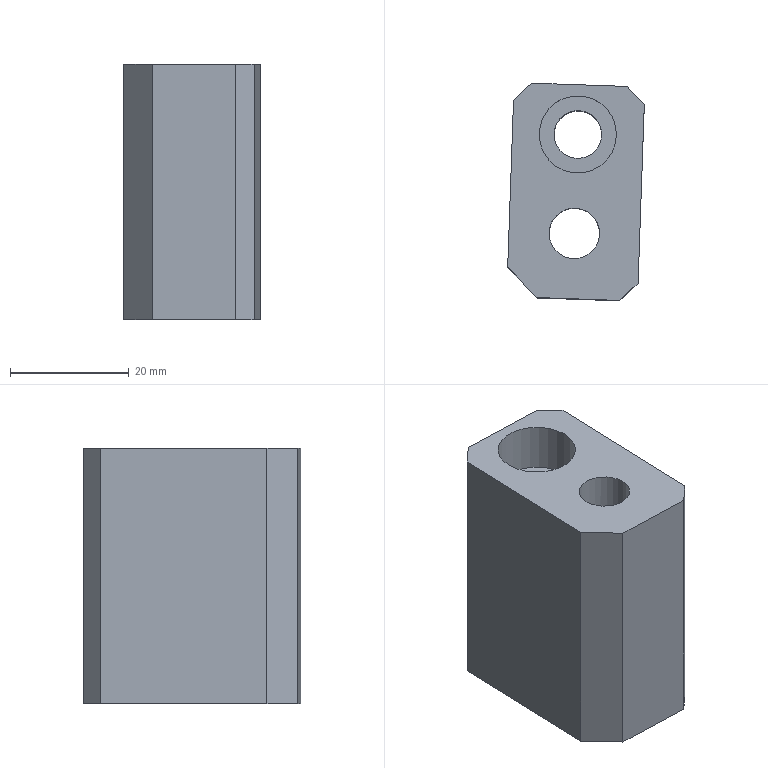Part | NX | features PH-11 2 | 1 solid | 16 faces | box 22.964 x 36.536 x 43 mm | volume 26468 mm3 | plane 12 | cylinder 4 | commonest cylinder face diameters 8.001 x1 8.5 x1 13 x1 14.5 x1
STEP:
#1=CARTESIAN_POINT('',(3338.766,-906.707,945.716));
#2=VERTEX_POINT('',#1);
#3=CARTESIAN_POINT('',(3332.266,-906.707,945.716));
#4=DIRECTION('',(0.,0.,1.));
#5=DIRECTION('',(1.,0.,0.));
#6=AXIS2_PLACEMENT_3D('',#3,#4,#5);
#7=CIRCLE('',#6,6.5);
#8=EDGE_CURVE('',#2,#2,#7,.F.);
#9=ORIENTED_EDGE('',*,*,#8,.T.);
#10=EDGE_LOOP('',(#9));
#11=FACE_BOUND('',#10,.T.);
#12=CARTESIAN_POINT('',(3335.932,-923.495,945.716));
#13=VERTEX_POINT('',#12);
#14=CARTESIAN_POINT('',(3331.685,-923.347,945.716));
#15=DIRECTION('',(0.,0.,-1.));
#16=DIRECTION('',(0.9994,-0.0349,0.));
#17=AXIS2_PLACEMENT_3D('',#14,#15,#16);
#18=CIRCLE('',#17,4.25);
#19=EDGE_CURVE('',#13,#13,#18,.T.);
#20=ORIENTED_EDGE('',*,*,#19,.T.);
#21=EDGE_LOOP('',(#20));
#22=FACE_BOUND('',#21,.T.);
#23=CARTESIAN_POINT('',(3321.459,-900.977,945.716));
#24=VERTEX_POINT('',#23);
#25=CARTESIAN_POINT('',(3320.482,-928.96,945.716));
#26=VERTEX_POINT('',#25);
#27=CARTESIAN_POINT('',(3320.936,-915.967,945.716));
#28=DIRECTION('',(-0.0349,-0.9994,0.));
#29=VECTOR('',#28,1000.);
#30=LINE('',#27,#29);
#31=EDGE_CURVE('',#24,#26,#30,.T.);
#32=ORIENTED_EDGE('',*,*,#31,.T.);
#33=CARTESIAN_POINT('',(3325.304,-934.131,945.716));
#34=VERTEX_POINT('',#33);
#35=CARTESIAN_POINT('',(3319.517,-927.925,945.716));
#36=DIRECTION('',(-0.682,0.7314,0.));
#37=VECTOR('',#36,1000.);
#38=LINE('',#35,#37);
#39=EDGE_CURVE('',#26,#34,#38,.F.);
#40=ORIENTED_EDGE('',*,*,#39,.T.);
#41=CARTESIAN_POINT('',(3339.296,-934.62,945.716));
#42=VERTEX_POINT('',#41);
#43=CARTESIAN_POINT('',(3331.301,-934.34,945.716));
#44=DIRECTION('',(0.9994,-0.0349,0.));
#45=VECTOR('',#44,1000.);
#46=LINE('',#43,#45);
#47=EDGE_CURVE('',#34,#42,#46,.T.);
#48=ORIENTED_EDGE('',*,*,#47,.T.);
#49=CARTESIAN_POINT('',(3342.399,-931.726,945.716));
#50=VERTEX_POINT('',#49);
#51=CARTESIAN_POINT('',(3344.467,-929.797,945.716));
#52=DIRECTION('',(0.7314,0.682,0.));
#53=VECTOR('',#52,1000.);
#54=LINE('',#51,#53);
#55=EDGE_CURVE('',#50,#42,#54,.F.);
#56=ORIENTED_EDGE('',*,*,#55,.F.);
#57=CARTESIAN_POINT('',(3343.446,-901.744,945.716));
#58=VERTEX_POINT('',#57);
#59=CARTESIAN_POINT('',(3342.922,-916.735,945.716));
#60=DIRECTION('',(0.0349,0.9994,0.));
#61=VECTOR('',#60,1000.);
#62=LINE('',#59,#61);
#63=EDGE_CURVE('',#50,#58,#62,.T.);
#64=ORIENTED_EDGE('',*,*,#63,.T.);
#65=CARTESIAN_POINT('',(3340.552,-898.641,945.716));
#66=VERTEX_POINT('',#65);
#67=CARTESIAN_POINT('',(3345.375,-903.813,945.716));
#68=DIRECTION('',(-0.682,0.7314,0.));
#69=VECTOR('',#68,1000.);
#70=LINE('',#67,#69);
#71=EDGE_CURVE('',#66,#58,#70,.F.);
#72=ORIENTED_EDGE('',*,*,#71,.F.);
#73=CARTESIAN_POINT('',(3324.562,-898.083,945.716));
#74=VERTEX_POINT('',#73);
#75=CARTESIAN_POINT('',(3332.557,-898.362,945.716));
#76=DIRECTION('',(-0.9994,0.0349,0.));
#77=VECTOR('',#76,1000.);
#78=LINE('',#75,#77);
#79=EDGE_CURVE('',#66,#74,#78,.T.);
#80=ORIENTED_EDGE('',*,*,#79,.T.);
#81=CARTESIAN_POINT('',(3319.39,-902.906,945.716));
#82=DIRECTION('',(-0.7314,-0.682,0.));
#83=VECTOR('',#82,1000.);
#84=LINE('',#81,#83);
#85=EDGE_CURVE('',#24,#74,#84,.F.);
#86=ORIENTED_EDGE('',*,*,#85,.F.);
#87=EDGE_LOOP('',(#32,#40,#48,#56,#64,#72,#80,#86));
#88=FACE_BOUND('',#87,.T.);
#89=CARTESIAN_POINT('',(3331.929,-916.351,945.716));
#90=DIRECTION('',(0.,0.,1.));
#91=DIRECTION('',(0.9994,-0.0349,0.));
#92=AXIS2_PLACEMENT_3D('',#89,#90,#91);
#93=PLANE('',#92);
#94=ADVANCED_FACE('',(#11,#22,#88),#93,.T.);
#95=CARTESIAN_POINT('',(3324.562,-898.083,902.716));
#96=VERTEX_POINT('',#95);
#97=CARTESIAN_POINT('',(3340.552,-898.641,902.716));
#98=VERTEX_POINT('',#97);
#99=CARTESIAN_POINT('',(3332.557,-898.362,902.716));
#100=DIRECTION('',(0.9994,-0.0349,0.));
#101=VECTOR('',#100,1000.);
#102=LINE('',#99,#101);
#103=EDGE_CURVE('',#96,#98,#102,.T.);
#104=ORIENTED_EDGE('',*,*,#103,.F.);
#105=CARTESIAN_POINT('',(3324.562,-898.083,920.716));
#106=DIRECTION('',(0.,0.,-1.));
#107=VECTOR('',#106,1000.);
#108=LINE('',#105,#107);
#109=EDGE_CURVE('',#74,#96,#108,.T.);
#110=ORIENTED_EDGE('',*,*,#109,.F.);
#111=ORIENTED_EDGE('',*,*,#79,.F.);
#112=CARTESIAN_POINT('',(3340.552,-898.641,920.716));
#113=DIRECTION('',(0.,0.,1.));
#114=VECTOR('',#113,1000.);
#115=LINE('',#112,#114);
#116=EDGE_CURVE('',#98,#66,#115,.T.);
#117=ORIENTED_EDGE('',*,*,#116,.F.);
#118=EDGE_LOOP('',(#104,#110,#111,#117));
#119=FACE_BOUND('',#118,.T.);
#120=CARTESIAN_POINT('',(3332.557,-898.362,920.716));
#121=DIRECTION('',(0.0349,0.9994,0.));
#122=DIRECTION('',(0.,0.,-1.));
#123=AXIS2_PLACEMENT_3D('',#120,#121,#122);
#124=PLANE('',#123);
#125=ADVANCED_FACE('',(#119),#124,.T.);
#126=CARTESIAN_POINT('',(3320.482,-928.96,902.716));
#127=VERTEX_POINT('',#126);
#128=CARTESIAN_POINT('',(3321.459,-900.977,902.716));
#129=VERTEX_POINT('',#128);
#130=CARTESIAN_POINT('',(3320.936,-915.967,902.716));
#131=DIRECTION('',(0.0349,0.9994,0.));
#132=VECTOR('',#131,1000.);
#133=LINE('',#130,#132);
#134=EDGE_CURVE('',#127,#129,#133,.T.);
#135=ORIENTED_EDGE('',*,*,#134,.F.);
#136=CARTESIAN_POINT('',(3320.482,-928.96,920.716));
#137=DIRECTION('',(0.,0.,1.));
#138=VECTOR('',#137,1000.);
#139=LINE('',#136,#138);
#140=EDGE_CURVE('',#127,#26,#139,.T.);
#141=ORIENTED_EDGE('',*,*,#140,.T.);
#142=ORIENTED_EDGE('',*,*,#31,.F.);
#143=CARTESIAN_POINT('',(3321.459,-900.977,920.716));
#144=DIRECTION('',(0.,0.,1.));
#145=VECTOR('',#144,1000.);
#146=LINE('',#143,#145);
#147=EDGE_CURVE('',#129,#24,#146,.T.);
#148=ORIENTED_EDGE('',*,*,#147,.F.);
#149=EDGE_LOOP('',(#135,#141,#142,#148));
#150=FACE_BOUND('',#149,.T.);
#151=CARTESIAN_POINT('',(3320.936,-915.967,920.716));
#152=DIRECTION('',(-0.9994,0.0349,0.));
#153=DIRECTION('',(0.,0.,1.));
#154=AXIS2_PLACEMENT_3D('',#151,#152,#153);
#155=PLANE('',#154);
#156=ADVANCED_FACE('',(#150),#155,.T.);
#157=ORIENTED_EDGE('',*,*,#47,.F.);
#158=CARTESIAN_POINT('',(3325.304,-934.131,902.716));
#159=VERTEX_POINT('',#158);
#160=CARTESIAN_POINT('',(3325.304,-934.131,920.716));
#161=DIRECTION('',(0.,0.,-1.));
#162=VECTOR('',#161,1000.);
#163=LINE('',#160,#162);
#164=EDGE_CURVE('',#34,#159,#163,.T.);
#165=ORIENTED_EDGE('',*,*,#164,.T.);
#166=CARTESIAN_POINT('',(3339.296,-934.62,902.716));
#167=VERTEX_POINT('',#166);
#168=CARTESIAN_POINT('',(3331.301,-934.34,902.716));
#169=DIRECTION('',(-0.9994,0.0349,0.));
#170=VECTOR('',#169,1000.);
#171=LINE('',#168,#170);
#172=EDGE_CURVE('',#167,#159,#171,.T.);
#173=ORIENTED_EDGE('',*,*,#172,.F.);
#174=CARTESIAN_POINT('',(3339.296,-934.62,920.716));
#175=DIRECTION('',(0.,0.,-1.));
#176=VECTOR('',#175,1000.);
#177=LINE('',#174,#176);
#178=EDGE_CURVE('',#42,#167,#177,.T.);
#179=ORIENTED_EDGE('',*,*,#178,.F.);
#180=EDGE_LOOP('',(#157,#165,#173,#179));
#181=FACE_BOUND('',#180,.T.);
#182=CARTESIAN_POINT('',(3331.301,-934.34,920.716));
#183=DIRECTION('',(-0.0349,-0.9994,0.));
#184=DIRECTION('',(0.,0.,1.));
#185=AXIS2_PLACEMENT_3D('',#182,#183,#184);
#186=PLANE('',#185);
#187=ADVANCED_FACE('',(#181),#186,.T.);
#188=CARTESIAN_POINT('',(3328.265,-906.707,902.716));
#189=VERTEX_POINT('',#188);
#190=CARTESIAN_POINT('',(3332.266,-906.707,902.716));
#191=DIRECTION('',(0.,0.,-1.));
#192=DIRECTION('',(-1.,0.,0.));
#193=AXIS2_PLACEMENT_3D('',#190,#191,#192);
#194=CIRCLE('',#193,4.);
#195=EDGE_CURVE('',#189,#189,#194,.T.);
#196=ORIENTED_EDGE('',*,*,#195,.F.);
#197=EDGE_LOOP('',(#196));
#198=FACE_BOUND('',#197,.T.);
#199=CARTESIAN_POINT('',(3324.435,-923.347,902.716));
#200=VERTEX_POINT('',#199);
#201=CARTESIAN_POINT('',(3331.685,-923.347,902.716));
#202=DIRECTION('',(0.,0.,-1.));
#203=DIRECTION('',(-1.,0.,0.));
#204=AXIS2_PLACEMENT_3D('',#201,#202,#203);
#205=CIRCLE('',#204,7.25);
#206=EDGE_CURVE('',#200,#200,#205,.T.);
#207=ORIENTED_EDGE('',*,*,#206,.F.);
#208=EDGE_LOOP('',(#207));
#209=FACE_BOUND('',#208,.T.);
#210=ORIENTED_EDGE('',*,*,#172,.T.);
#211=CARTESIAN_POINT('',(3319.517,-927.925,902.716));
#212=DIRECTION('',(0.682,-0.7314,0.));
#213=VECTOR('',#212,1000.);
#214=LINE('',#211,#213);
#215=EDGE_CURVE('',#159,#127,#214,.F.);
#216=ORIENTED_EDGE('',*,*,#215,.T.);
#217=ORIENTED_EDGE('',*,*,#134,.T.);
#218=CARTESIAN_POINT('',(3321.459,-900.977,902.716));
#219=DIRECTION('',(0.7314,0.682,0.));
#220=VECTOR('',#219,1000.);
#221=LINE('',#218,#220);
#222=EDGE_CURVE('',#96,#129,#221,.F.);
#223=ORIENTED_EDGE('',*,*,#222,.F.);
#224=ORIENTED_EDGE('',*,*,#103,.T.);
#225=CARTESIAN_POINT('',(3343.446,-901.744,902.716));
#226=VERTEX_POINT('',#225);
#227=CARTESIAN_POINT('',(3340.552,-898.641,902.716));
#228=DIRECTION('',(0.682,-0.7314,0.));
#229=VECTOR('',#228,1000.);
#230=LINE('',#227,#229);
#231=EDGE_CURVE('',#226,#98,#230,.F.);
#232=ORIENTED_EDGE('',*,*,#231,.F.);
#233=CARTESIAN_POINT('',(3342.399,-931.726,902.716));
#234=VERTEX_POINT('',#233);
#235=CARTESIAN_POINT('',(3342.922,-916.735,902.716));
#236=DIRECTION('',(-0.0349,-0.9994,0.));
#237=VECTOR('',#236,1000.);
#238=LINE('',#235,#237);
#239=EDGE_CURVE('',#226,#234,#238,.T.);
#240=ORIENTED_EDGE('',*,*,#239,.T.);
#241=CARTESIAN_POINT('',(3342.399,-931.726,902.716));
#242=DIRECTION('',(-0.7314,-0.682,0.));
#243=VECTOR('',#242,1000.);
#244=LINE('',#241,#243);
#245=EDGE_CURVE('',#167,#234,#244,.F.);
#246=ORIENTED_EDGE('',*,*,#245,.F.);
#247=EDGE_LOOP('',(#210,#216,#217,#223,#224,#232,#240,#246));
#248=FACE_BOUND('',#247,.T.);
#249=CARTESIAN_POINT('',(3331.929,-916.351,902.716));
#250=DIRECTION('',(0.,0.,-1.));
#251=DIRECTION('',(-0.9994,0.0349,0.));
#252=AXIS2_PLACEMENT_3D('',#249,#250,#251);
#253=PLANE('',#252);
#254=ADVANCED_FACE('',(#198,#209,#248),#253,.T.);
#255=ORIENTED_EDGE('',*,*,#239,.F.);
#256=CARTESIAN_POINT('',(3343.446,-901.744,920.716));
#257=DIRECTION('',(0.,0.,-1.));
#258=VECTOR('',#257,1000.);
#259=LINE('',#256,#258);
#260=EDGE_CURVE('',#58,#226,#259,.T.);
#261=ORIENTED_EDGE('',*,*,#260,.F.);
#262=ORIENTED_EDGE('',*,*,#63,.F.);
#263=CARTESIAN_POINT('',(3342.399,-931.726,920.716));
#264=DIRECTION('',(0.,0.,1.));
#265=VECTOR('',#264,1000.);
#266=LINE('',#263,#265);
#267=EDGE_CURVE('',#234,#50,#266,.T.);
#268=ORIENTED_EDGE('',*,*,#267,.F.);
#269=EDGE_LOOP('',(#255,#261,#262,#268));
#270=FACE_BOUND('',#269,.T.);
#271=CARTESIAN_POINT('',(3342.922,-916.735,920.716));
#272=DIRECTION('',(0.9994,-0.0349,0.));
#273=DIRECTION('',(0.,0.,-1.));
#274=AXIS2_PLACEMENT_3D('',#271,#272,#273);
#275=PLANE('',#274);
#276=ADVANCED_FACE('',(#270),#275,.T.);
#277=ORIENTED_EDGE('',*,*,#245,.T.);
#278=ORIENTED_EDGE('',*,*,#267,.T.);
#279=ORIENTED_EDGE('',*,*,#55,.T.);
#280=ORIENTED_EDGE('',*,*,#178,.T.);
#281=EDGE_LOOP('',(#277,#278,#279,#280));
#282=FACE_BOUND('',#281,.T.);
#283=CARTESIAN_POINT('',(3342.399,-931.726,920.716));
#284=DIRECTION('',(-0.682,0.7314,0.));
#285=DIRECTION('',(0.7314,0.682,0.));
#286=AXIS2_PLACEMENT_3D('',#283,#284,#285);
#287=PLANE('',#286);
#288=ADVANCED_FACE('',(#282),#287,.F.);
#289=ORIENTED_EDGE('',*,*,#231,.T.);
#290=ORIENTED_EDGE('',*,*,#116,.T.);
#291=ORIENTED_EDGE('',*,*,#71,.T.);
#292=ORIENTED_EDGE('',*,*,#260,.T.);
#293=EDGE_LOOP('',(#289,#290,#291,#292));
#294=FACE_BOUND('',#293,.T.);
#295=CARTESIAN_POINT('',(3340.552,-898.641,920.716));
#296=DIRECTION('',(-0.7314,-0.682,0.));
#297=DIRECTION('',(-0.682,0.7314,0.));
#298=AXIS2_PLACEMENT_3D('',#295,#296,#297);
#299=PLANE('',#298);
#300=ADVANCED_FACE('',(#294),#299,.F.);
#301=ORIENTED_EDGE('',*,*,#222,.T.);
#302=ORIENTED_EDGE('',*,*,#147,.T.);
#303=ORIENTED_EDGE('',*,*,#85,.T.);
#304=ORIENTED_EDGE('',*,*,#109,.T.);
#305=EDGE_LOOP('',(#301,#302,#303,#304));
#306=FACE_BOUND('',#305,.T.);
#307=CARTESIAN_POINT('',(3321.459,-900.977,920.716));
#308=DIRECTION('',(0.682,-0.7314,0.));
#309=DIRECTION('',(-0.7314,-0.682,0.));
#310=AXIS2_PLACEMENT_3D('',#307,#308,#309);
#311=PLANE('',#310);
#312=ADVANCED_FACE('',(#306),#311,.F.);
#313=CARTESIAN_POINT('',(3335.935,-923.347,913.716));
#314=VERTEX_POINT('',#313);
#315=CARTESIAN_POINT('',(3331.685,-923.347,913.716));
#316=DIRECTION('',(0.,0.,1.));
#317=DIRECTION('',(1.,0.,0.));
#318=AXIS2_PLACEMENT_3D('',#315,#316,#317);
#319=CIRCLE('',#318,4.25);
#320=EDGE_CURVE('',#314,#314,#319,.F.);
#321=ORIENTED_EDGE('',*,*,#320,.F.);
#322=EDGE_LOOP('',(#321));
#323=FACE_BOUND('',#322,.T.);
#324=CARTESIAN_POINT('',(3338.935,-923.347,913.716));
#325=VERTEX_POINT('',#324);
#326=CARTESIAN_POINT('',(3331.685,-923.347,913.716));
#327=DIRECTION('',(0.,0.,1.));
#328=DIRECTION('',(1.,0.,0.));
#329=AXIS2_PLACEMENT_3D('',#326,#327,#328);
#330=CIRCLE('',#329,7.25);
#331=EDGE_CURVE('',#325,#325,#330,.F.);
#332=ORIENTED_EDGE('',*,*,#331,.T.);
#333=EDGE_LOOP('',(#332));
#334=FACE_BOUND('',#333,.T.);
#335=CARTESIAN_POINT('',(3331.685,-923.347,913.716));
#336=DIRECTION('',(0.,0.,1.));
#337=DIRECTION('',(0.9994,-0.0349,0.));
#338=AXIS2_PLACEMENT_3D('',#335,#336,#337);
#339=PLANE('',#338);
#340=ADVANCED_FACE('',(#323,#334),#339,.F.);
#341=ORIENTED_EDGE('',*,*,#206,.T.);
#342=EDGE_LOOP('',(#341));
#343=FACE_BOUND('',#342,.T.);
#344=ORIENTED_EDGE('',*,*,#331,.F.);
#345=EDGE_LOOP('',(#344));
#346=FACE_BOUND('',#345,.T.);
#347=CARTESIAN_POINT('',(3331.685,-923.347,931.716));
#348=DIRECTION('',(0.,0.,-1.));
#349=DIRECTION('',(0.9994,-0.0349,0.));
#350=AXIS2_PLACEMENT_3D('',#347,#348,#349);
#351=CYLINDRICAL_SURFACE('',#350,7.25);
#352=ADVANCED_FACE('',(#343,#346),#351,.F.);
#353=ORIENTED_EDGE('',*,*,#19,.F.);
#354=EDGE_LOOP('',(#353));
#355=FACE_BOUND('',#354,.T.);
#356=ORIENTED_EDGE('',*,*,#320,.T.);
#357=EDGE_LOOP('',(#356));
#358=FACE_BOUND('',#357,.T.);
#359=CARTESIAN_POINT('',(3331.685,-923.347,946.716));
#360=DIRECTION('',(0.,0.,-1.));
#361=DIRECTION('',(0.9994,-0.0349,0.));
#362=AXIS2_PLACEMENT_3D('',#359,#360,#361);
#363=CYLINDRICAL_SURFACE('',#362,4.25);
#364=ADVANCED_FACE('',(#355,#358),#363,.F.);
#365=ORIENTED_EDGE('',*,*,#195,.T.);
#366=EDGE_LOOP('',(#365));
#367=FACE_BOUND('',#366,.T.);
#368=CARTESIAN_POINT('',(3328.265,-906.707,937.516));
#369=VERTEX_POINT('',#368);
#370=CARTESIAN_POINT('',(3332.266,-906.707,937.516));
#371=DIRECTION('',(0.,0.,-1.));
#372=DIRECTION('',(-1.,0.,0.));
#373=AXIS2_PLACEMENT_3D('',#370,#371,#372);
#374=CIRCLE('',#373,4.);
#375=EDGE_CURVE('',#369,#369,#374,.T.);
#376=ORIENTED_EDGE('',*,*,#375,.F.);
#377=EDGE_LOOP('',(#376));
#378=FACE_BOUND('',#377,.T.);
#379=CARTESIAN_POINT('',(3332.266,-906.707,945.716));
#380=DIRECTION('',(0.,0.,-1.));
#381=DIRECTION('',(1.,0.,0.));
#382=AXIS2_PLACEMENT_3D('',#379,#380,#381);
#383=CYLINDRICAL_SURFACE('',#382,4.);
#384=ADVANCED_FACE('',(#367,#378),#383,.F.);
#385=ORIENTED_EDGE('',*,*,#375,.T.);
#386=EDGE_LOOP('',(#385));
#387=FACE_BOUND('',#386,.T.);
#388=CARTESIAN_POINT('',(3325.766,-906.707,937.516));
#389=VERTEX_POINT('',#388);
#390=CARTESIAN_POINT('',(3332.266,-906.707,937.516));
#391=DIRECTION('',(0.,0.,-1.));
#392=DIRECTION('',(-1.,0.,0.));
#393=AXIS2_PLACEMENT_3D('',#390,#391,#392);
#394=CIRCLE('',#393,6.5);
#395=EDGE_CURVE('',#389,#389,#394,.T.);
#396=ORIENTED_EDGE('',*,*,#395,.F.);
#397=EDGE_LOOP('',(#396));
#398=FACE_BOUND('',#397,.T.);
#399=CARTESIAN_POINT('',(3332.266,-906.707,937.516));
#400=DIRECTION('',(0.,0.,-1.));
#401=DIRECTION('',(-1.,0.,0.));
#402=AXIS2_PLACEMENT_3D('',#399,#400,#401);
#403=PLANE('',#402);
#404=ADVANCED_FACE('',(#387,#398),#403,.F.);
#405=ORIENTED_EDGE('',*,*,#395,.T.);
#406=EDGE_LOOP('',(#405));
#407=FACE_BOUND('',#406,.T.);
#408=ORIENTED_EDGE('',*,*,#8,.F.);
#409=EDGE_LOOP('',(#408));
#410=FACE_BOUND('',#409,.T.);
#411=CARTESIAN_POINT('',(3332.266,-906.707,945.716));
#412=DIRECTION('',(0.,0.,-1.));
#413=DIRECTION('',(1.,0.,0.));
#414=AXIS2_PLACEMENT_3D('',#411,#412,#413);
#415=CYLINDRICAL_SURFACE('',#414,6.5);
#416=ADVANCED_FACE('',(#407,#410),#415,.F.);
#417=ORIENTED_EDGE('',*,*,#39,.F.);
#418=ORIENTED_EDGE('',*,*,#140,.F.);
#419=ORIENTED_EDGE('',*,*,#215,.F.);
#420=ORIENTED_EDGE('',*,*,#164,.F.);
#421=EDGE_LOOP('',(#417,#418,#419,#420));
#422=FACE_BOUND('',#421,.T.);
#423=CARTESIAN_POINT('',(3325.304,-934.131,920.716));
#424=DIRECTION('',(0.7314,0.682,0.));
#425=DIRECTION('',(0.,0.,-1.));
#426=AXIS2_PLACEMENT_3D('',#423,#424,#425);
#427=PLANE('',#426);
#428=ADVANCED_FACE('',(#422),#427,.F.);
#429=CLOSED_SHELL('',(#94,#125,#156,#187,#254,#276,#288,#300,#312,#340,#352,#364,#384,#404,#416,#428));
#430=MANIFOLD_SOLID_BREP('',#429);
#431=(LENGTH_UNIT()NAMED_UNIT(*)SI_UNIT(.MILLI.,.METRE.));
#432=UNCERTAINTY_MEASURE_WITH_UNIT(LENGTH_MEASURE(0.00001),#431,'','');
#433=(NAMED_UNIT(*)PLANE_ANGLE_UNIT()SI_UNIT($,.RADIAN.));
#434=(NAMED_UNIT(*)SI_UNIT($,.STERADIAN.)SOLID_ANGLE_UNIT());
#435=(GEOMETRIC_REPRESENTATION_CONTEXT(3)GLOBAL_UNCERTAINTY_ASSIGNED_CONTEXT((#432))GLOBAL_UNIT_ASSIGNED_CONTEXT((#431,#433,#434))REPRESENTATION_CONTEXT('',''));
#436=ADVANCED_BREP_SHAPE_REPRESENTATION('',(#430),#435);